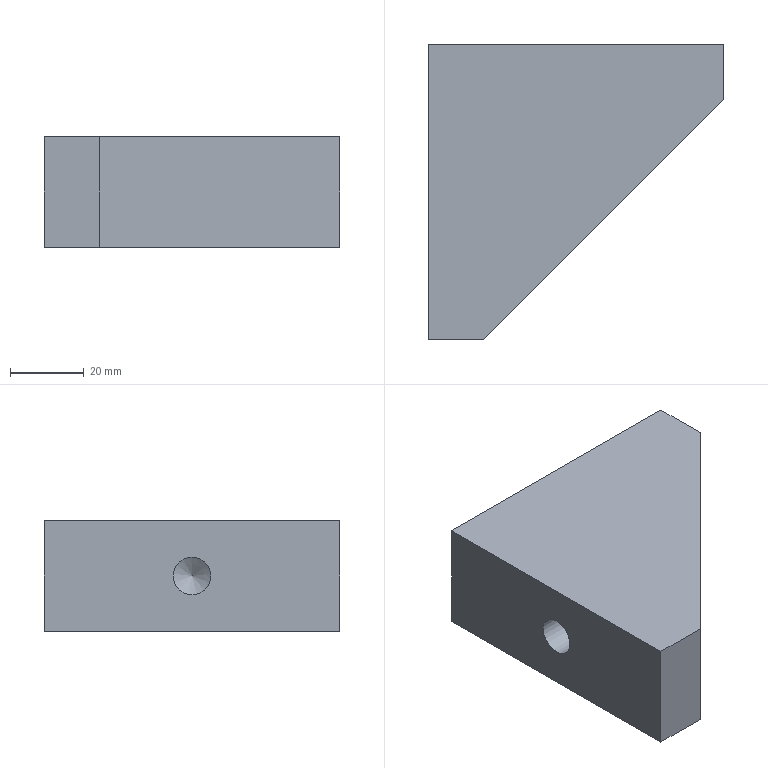Part | NX | features stifener1 2 | 1 solid | 11 faces | volume 123670 mm3 | plane 7 | cone 2 | cylinder 2 | commonest cylinder face diameters 10.2 x2